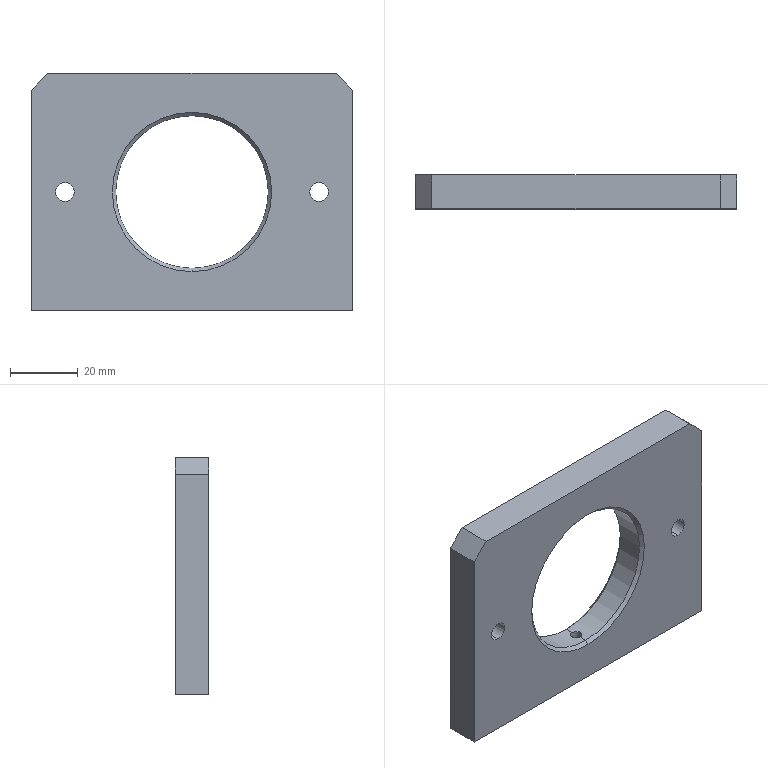Part | STEP file | 1 solid | 42 faces | box 95 x 10 x 70 mm | volume 48778 mm3 | cylinder 20 | cone 12 | plane 10 | commonest cylinder face diameters 3.3 x6 5 x4 5.5 x4 8 x4 45 x2